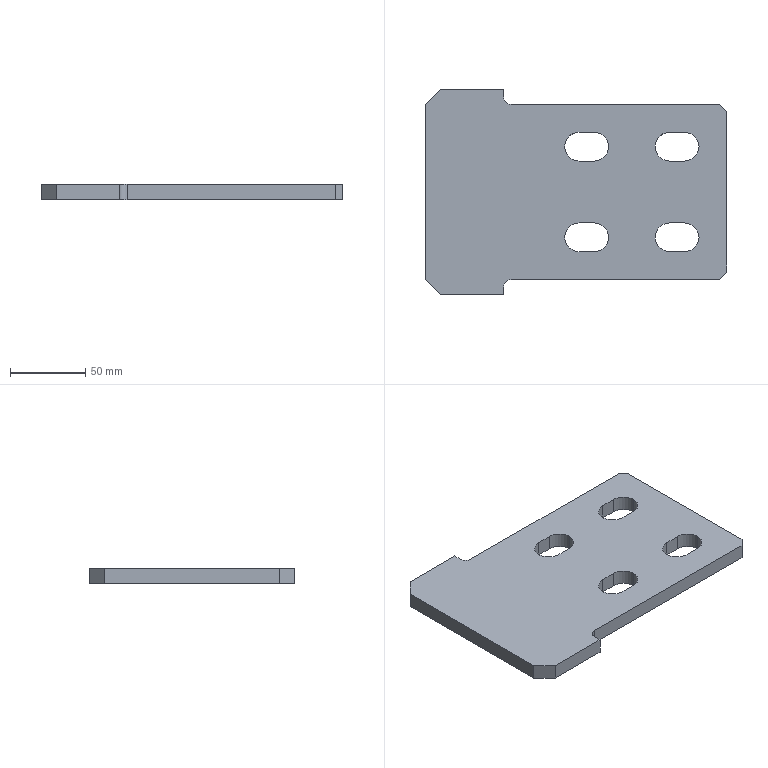Part | STEP file | 筋Plate-150×75-150-30度 | 1 solid | 36 faces | box 200 x 136 x 10 mm | volume 222316 mm3 | plane 22 | cylinder 14 | commonest cylinder face diameters 19 x12 10 x2